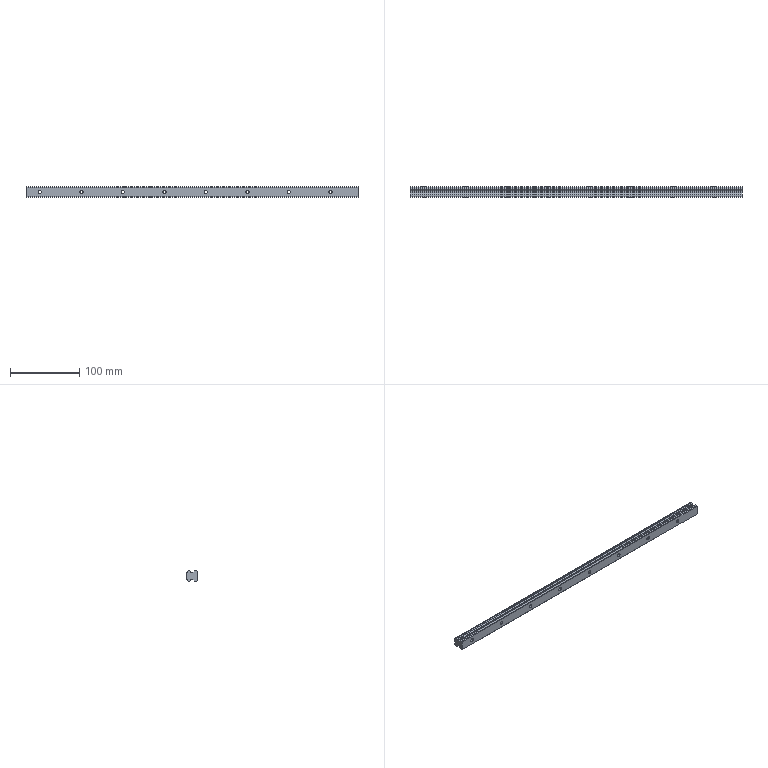Part | STEP file | 001-008-Rail_HGR15R04801_20_0 | 1 solid | 114 faces | box 480 x 15 x 15 mm | volume 88626 mm3 | cone 48 | cylinder 36 | plane 30 | commonest cylinder face diameters 4.5 x16 7.5 x16 3.2 x4